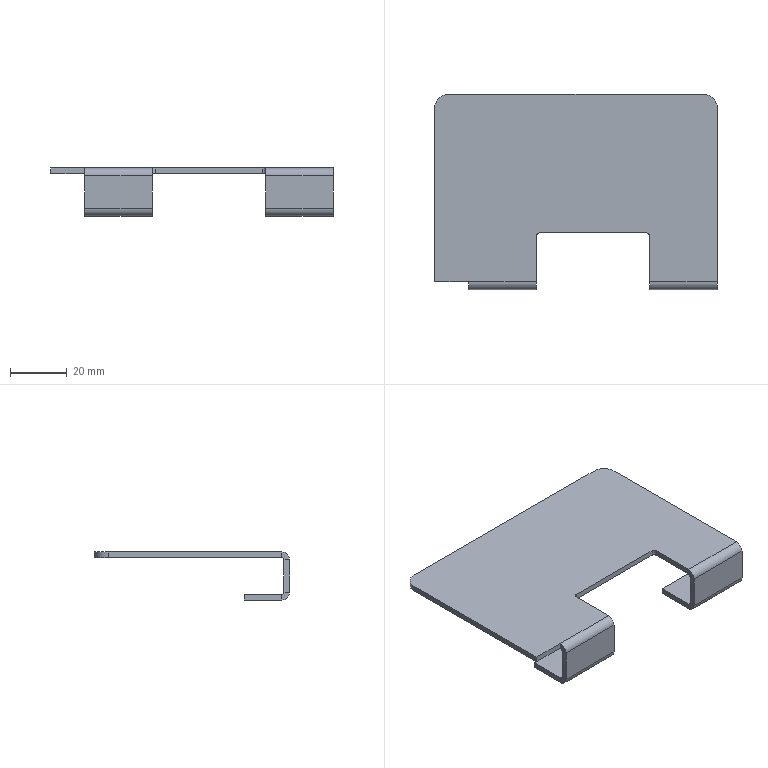Part | STEP file | H_ND25042-01-JG-002-BJ | 1 solid | 47 faces | box 100 x 69 x 17 mm | volume 14755 mm3 | plane 35 | cylinder 12 | commonest cylinder face diameters 1.473 x4 5.473 x4 2 x2 10 x2